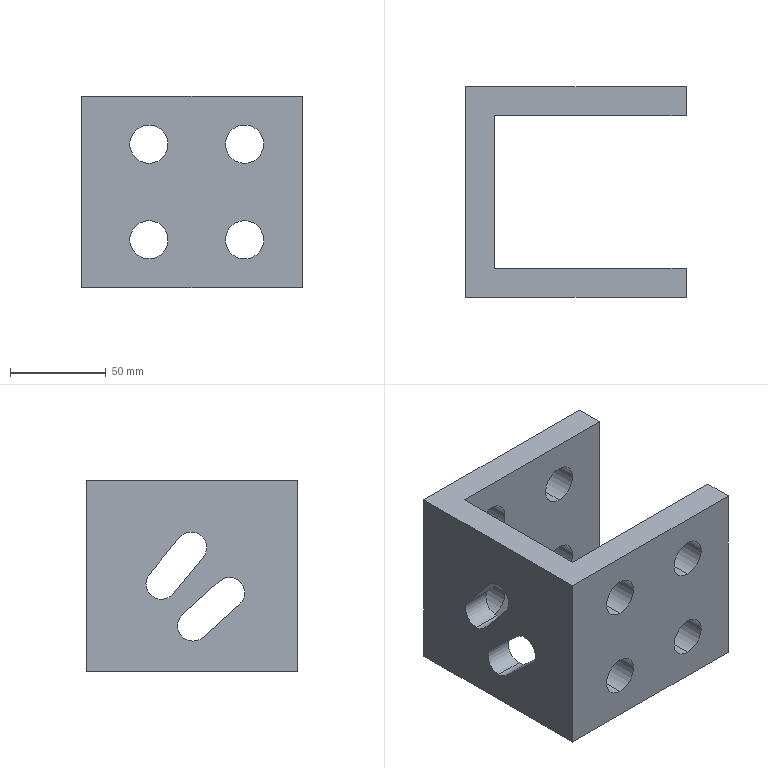Part | SolidWorks | features ICE 2, Extrusion 1 | 1 solid | 36 faces | box 115 x 110 x 100 mm | volume 409059 mm3 | cylinder 22 | plane 14 | commonest cylinder face diameters 20 x16 16.048 x3 16.141 x3
STEP:
#1=CARTESIAN_POINT('',(-15.,39.555,15.955));
#2=VERTEX_POINT('',#1);
#3=CARTESIAN_POINT('',(-15.,44.934,29.933));
#4=VERTEX_POINT('',#3);
#5=CARTESIAN_POINT('',(-15.,39.555,23.979));
#6=DIRECTION('',(1.,0.,0.));
#7=DIRECTION('',(0.,0.,-1.));
#8=AXIS2_PLACEMENT_3D('',#5,#6,#7);
#9=CIRCLE('',#8,8.024);
#10=EDGE_CURVE('',#2,#4,#9,.T.);
#11=ORIENTED_EDGE('',*,*,#10,.F.);
#12=CARTESIAN_POINT('',(0.,39.555,15.955));
#13=VERTEX_POINT('',#12);
#14=CARTESIAN_POINT('',(-500.,39.555,15.955));
#15=DIRECTION('',(1.,0.,0.));
#16=VECTOR('',#15,1000.);
#17=LINE('',#14,#16);
#18=EDGE_CURVE('',#2,#13,#17,.T.);
#19=ORIENTED_EDGE('',*,*,#18,.T.);
#20=CARTESIAN_POINT('',(0.,44.934,29.933));
#21=VERTEX_POINT('',#20);
#22=CARTESIAN_POINT('',(0.,39.555,23.979));
#23=DIRECTION('',(1.,0.,0.));
#24=DIRECTION('',(0.,0.,-1.));
#25=AXIS2_PLACEMENT_3D('',#22,#23,#24);
#26=CIRCLE('',#25,8.024);
#27=EDGE_CURVE('',#13,#21,#26,.T.);
#28=ORIENTED_EDGE('',*,*,#27,.T.);
#29=CARTESIAN_POINT('',(-500.,44.934,29.933));
#30=DIRECTION('',(1.,0.,0.));
#31=VECTOR('',#30,1000.);
#32=LINE('',#29,#31);
#33=EDGE_CURVE('',#4,#21,#32,.T.);
#34=ORIENTED_EDGE('',*,*,#33,.F.);
#35=EDGE_LOOP('',(#11,#19,#28,#34));
#36=FACE_OUTER_BOUND('',#35,.T.);
#37=CARTESIAN_POINT('',(-500.,39.555,23.979));
#38=DIRECTION('',(1.,0.,0.));
#39=DIRECTION('',(0.,0.,-1.));
#40=AXIS2_PLACEMENT_3D('',#37,#38,#39);
#41=CYLINDRICAL_SURFACE('',#40,8.024);
#42=ADVANCED_FACE('',(#36),#41,.F.);
#43=CARTESIAN_POINT('',(-15.,56.004,37.787));
#44=VERTEX_POINT('',#43);
#45=CARTESIAN_POINT('',(-15.,62.246,50.974));
#46=VERTEX_POINT('',#45);
#47=CARTESIAN_POINT('',(-15.,56.004,45.857));
#48=DIRECTION('',(1.,0.,0.));
#49=DIRECTION('',(0.,0.,-1.));
#50=AXIS2_PLACEMENT_3D('',#47,#48,#49);
#51=CIRCLE('',#50,8.071);
#52=EDGE_CURVE('',#44,#46,#51,.T.);
#53=ORIENTED_EDGE('',*,*,#52,.F.);
#54=CARTESIAN_POINT('',(0.,56.004,37.787));
#55=VERTEX_POINT('',#54);
#56=CARTESIAN_POINT('',(-500.,56.004,37.787));
#57=DIRECTION('',(1.,0.,0.));
#58=VECTOR('',#57,1000.);
#59=LINE('',#56,#58);
#60=EDGE_CURVE('',#44,#55,#59,.T.);
#61=ORIENTED_EDGE('',*,*,#60,.T.);
#62=CARTESIAN_POINT('',(0.,62.246,50.974));
#63=VERTEX_POINT('',#62);
#64=CARTESIAN_POINT('',(0.,56.004,45.857));
#65=DIRECTION('',(1.,0.,0.));
#66=DIRECTION('',(0.,0.,-1.));
#67=AXIS2_PLACEMENT_3D('',#64,#65,#66);
#68=CIRCLE('',#67,8.071);
#69=EDGE_CURVE('',#55,#63,#68,.T.);
#70=ORIENTED_EDGE('',*,*,#69,.T.);
#71=CARTESIAN_POINT('',(-500.,62.246,50.974));
#72=DIRECTION('',(1.,0.,0.));
#73=VECTOR('',#72,1000.);
#74=LINE('',#71,#73);
#75=EDGE_CURVE('',#46,#63,#74,.T.);
#76=ORIENTED_EDGE('',*,*,#75,.F.);
#77=EDGE_LOOP('',(#53,#61,#70,#76));
#78=FACE_OUTER_BOUND('',#77,.T.);
#79=CARTESIAN_POINT('',(-500.,56.004,45.857));
#80=DIRECTION('',(1.,0.,0.));
#81=DIRECTION('',(0.,0.,-1.));
#82=AXIS2_PLACEMENT_3D('',#79,#80,#81);
#83=CYLINDRICAL_SURFACE('',#82,8.071);
#84=ADVANCED_FACE('',(#78),#83,.F.);
#85=CARTESIAN_POINT('',(70.,80.,15.));
#86=VERTEX_POINT('',#85);
#87=CARTESIAN_POINT('',(70.,80.,35.));
#88=VERTEX_POINT('',#87);
#89=CARTESIAN_POINT('',(70.,80.,25.));
#90=DIRECTION('',(0.,1.,0.));
#91=DIRECTION('',(0.,0.,1.));
#92=AXIS2_PLACEMENT_3D('',#89,#90,#91);
#93=CIRCLE('',#92,10.);
#94=EDGE_CURVE('',#86,#88,#93,.T.);
#95=ORIENTED_EDGE('',*,*,#94,.F.);
#96=CARTESIAN_POINT('',(70.,95.,15.));
#97=VERTEX_POINT('',#96);
#98=CARTESIAN_POINT('',(70.,-405.,15.));
#99=DIRECTION('',(0.,1.,0.));
#100=VECTOR('',#99,1000.);
#101=LINE('',#98,#100);
#102=EDGE_CURVE('',#86,#97,#101,.T.);
#103=ORIENTED_EDGE('',*,*,#102,.T.);
#104=CARTESIAN_POINT('',(70.,95.,35.));
#105=VERTEX_POINT('',#104);
#106=CARTESIAN_POINT('',(70.,95.,25.));
#107=DIRECTION('',(0.,1.,0.));
#108=DIRECTION('',(0.,0.,1.));
#109=AXIS2_PLACEMENT_3D('',#106,#107,#108);
#110=CIRCLE('',#109,10.);
#111=EDGE_CURVE('',#97,#105,#110,.T.);
#112=ORIENTED_EDGE('',*,*,#111,.T.);
#113=CARTESIAN_POINT('',(70.,-405.,35.));
#114=DIRECTION('',(0.,1.,0.));
#115=VECTOR('',#114,1000.);
#116=LINE('',#113,#115);
#117=EDGE_CURVE('',#88,#105,#116,.T.);
#118=ORIENTED_EDGE('',*,*,#117,.F.);
#119=EDGE_LOOP('',(#95,#103,#112,#118));
#120=FACE_OUTER_BOUND('',#119,.T.);
#121=CARTESIAN_POINT('',(70.,-405.,25.));
#122=DIRECTION('',(0.,1.,0.));
#123=DIRECTION('',(0.,0.,1.));
#124=AXIS2_PLACEMENT_3D('',#121,#122,#123);
#125=CYLINDRICAL_SURFACE('',#124,10.);
#126=ADVANCED_FACE('',(#120),#125,.F.);
#127=CARTESIAN_POINT('',(20.,80.,65.));
#128=VERTEX_POINT('',#127);
#129=CARTESIAN_POINT('',(20.,80.,85.));
#130=VERTEX_POINT('',#129);
#131=CARTESIAN_POINT('',(20.,80.,75.));
#132=DIRECTION('',(0.,1.,0.));
#133=DIRECTION('',(0.,0.,1.));
#134=AXIS2_PLACEMENT_3D('',#131,#132,#133);
#135=CIRCLE('',#134,10.);
#136=EDGE_CURVE('',#128,#130,#135,.T.);
#137=ORIENTED_EDGE('',*,*,#136,.F.);
#138=CARTESIAN_POINT('',(20.,95.,65.));
#139=VERTEX_POINT('',#138);
#140=CARTESIAN_POINT('',(20.,-405.,65.));
#141=DIRECTION('',(0.,1.,0.));
#142=VECTOR('',#141,1000.);
#143=LINE('',#140,#142);
#144=EDGE_CURVE('',#128,#139,#143,.T.);
#145=ORIENTED_EDGE('',*,*,#144,.T.);
#146=CARTESIAN_POINT('',(20.,95.,85.));
#147=VERTEX_POINT('',#146);
#148=CARTESIAN_POINT('',(20.,95.,75.));
#149=DIRECTION('',(0.,1.,0.));
#150=DIRECTION('',(0.,0.,1.));
#151=AXIS2_PLACEMENT_3D('',#148,#149,#150);
#152=CIRCLE('',#151,10.);
#153=EDGE_CURVE('',#139,#147,#152,.T.);
#154=ORIENTED_EDGE('',*,*,#153,.T.);
#155=CARTESIAN_POINT('',(20.,-405.,85.));
#156=DIRECTION('',(0.,1.,0.));
#157=VECTOR('',#156,1000.);
#158=LINE('',#155,#157);
#159=EDGE_CURVE('',#130,#147,#158,.T.);
#160=ORIENTED_EDGE('',*,*,#159,.F.);
#161=EDGE_LOOP('',(#137,#145,#154,#160));
#162=FACE_OUTER_BOUND('',#161,.T.);
#163=CARTESIAN_POINT('',(20.,-405.,75.));
#164=DIRECTION('',(0.,1.,0.));
#165=DIRECTION('',(0.,0.,1.));
#166=AXIS2_PLACEMENT_3D('',#163,#164,#165);
#167=CYLINDRICAL_SURFACE('',#166,10.);
#168=ADVANCED_FACE('',(#162),#167,.F.);
#169=CARTESIAN_POINT('',(70.,80.,65.));
#170=VERTEX_POINT('',#169);
#171=CARTESIAN_POINT('',(70.,80.,85.));
#172=VERTEX_POINT('',#171);
#173=CARTESIAN_POINT('',(70.,80.,75.));
#174=DIRECTION('',(0.,1.,0.));
#175=DIRECTION('',(0.,0.,1.));
#176=AXIS2_PLACEMENT_3D('',#173,#174,#175);
#177=CIRCLE('',#176,10.);
#178=EDGE_CURVE('',#170,#172,#177,.T.);
#179=ORIENTED_EDGE('',*,*,#178,.F.);
#180=CARTESIAN_POINT('',(70.,95.,65.));
#181=VERTEX_POINT('',#180);
#182=CARTESIAN_POINT('',(70.,-405.,65.));
#183=DIRECTION('',(0.,1.,0.));
#184=VECTOR('',#183,1000.);
#185=LINE('',#182,#184);
#186=EDGE_CURVE('',#170,#181,#185,.T.);
#187=ORIENTED_EDGE('',*,*,#186,.T.);
#188=CARTESIAN_POINT('',(70.,95.,85.));
#189=VERTEX_POINT('',#188);
#190=CARTESIAN_POINT('',(70.,95.,75.));
#191=DIRECTION('',(0.,1.,0.));
#192=DIRECTION('',(0.,0.,1.));
#193=AXIS2_PLACEMENT_3D('',#190,#191,#192);
#194=CIRCLE('',#193,10.);
#195=EDGE_CURVE('',#181,#189,#194,.T.);
#196=ORIENTED_EDGE('',*,*,#195,.T.);
#197=CARTESIAN_POINT('',(70.,-405.,85.));
#198=DIRECTION('',(0.,1.,0.));
#199=VECTOR('',#198,1000.);
#200=LINE('',#197,#199);
#201=EDGE_CURVE('',#172,#189,#200,.T.);
#202=ORIENTED_EDGE('',*,*,#201,.F.);
#203=EDGE_LOOP('',(#179,#187,#196,#202));
#204=FACE_OUTER_BOUND('',#203,.T.);
#205=CARTESIAN_POINT('',(70.,-405.,75.));
#206=DIRECTION('',(0.,1.,0.));
#207=DIRECTION('',(0.,0.,1.));
#208=AXIS2_PLACEMENT_3D('',#205,#206,#207);
#209=CYLINDRICAL_SURFACE('',#208,10.);
#210=ADVANCED_FACE('',(#204),#209,.F.);
#211=CARTESIAN_POINT('',(20.,80.,15.));
#212=VERTEX_POINT('',#211);
#213=CARTESIAN_POINT('',(20.,80.,35.));
#214=VERTEX_POINT('',#213);
#215=CARTESIAN_POINT('',(20.,80.,25.));
#216=DIRECTION('',(0.,1.,0.));
#217=DIRECTION('',(0.,0.,1.));
#218=AXIS2_PLACEMENT_3D('',#215,#216,#217);
#219=CIRCLE('',#218,10.);
#220=EDGE_CURVE('',#212,#214,#219,.T.);
#221=ORIENTED_EDGE('',*,*,#220,.F.);
#222=CARTESIAN_POINT('',(20.,95.,15.));
#223=VERTEX_POINT('',#222);
#224=CARTESIAN_POINT('',(20.,-405.,15.));
#225=DIRECTION('',(0.,1.,0.));
#226=VECTOR('',#225,1000.);
#227=LINE('',#224,#226);
#228=EDGE_CURVE('',#212,#223,#227,.T.);
#229=ORIENTED_EDGE('',*,*,#228,.T.);
#230=CARTESIAN_POINT('',(20.,95.,35.));
#231=VERTEX_POINT('',#230);
#232=CARTESIAN_POINT('',(20.,95.,25.));
#233=DIRECTION('',(0.,1.,0.));
#234=DIRECTION('',(0.,0.,1.));
#235=AXIS2_PLACEMENT_3D('',#232,#233,#234);
#236=CIRCLE('',#235,10.);
#237=EDGE_CURVE('',#223,#231,#236,.T.);
#238=ORIENTED_EDGE('',*,*,#237,.T.);
#239=CARTESIAN_POINT('',(20.,-405.,35.));
#240=DIRECTION('',(0.,1.,0.));
#241=VECTOR('',#240,1000.);
#242=LINE('',#239,#241);
#243=EDGE_CURVE('',#214,#231,#242,.T.);
#244=ORIENTED_EDGE('',*,*,#243,.F.);
#245=EDGE_LOOP('',(#221,#229,#238,#244));
#246=FACE_OUTER_BOUND('',#245,.T.);
#247=CARTESIAN_POINT('',(20.,-405.,25.));
#248=DIRECTION('',(0.,1.,0.));
#249=DIRECTION('',(0.,0.,1.));
#250=AXIS2_PLACEMENT_3D('',#247,#248,#249);
#251=CYLINDRICAL_SURFACE('',#250,10.);
#252=ADVANCED_FACE('',(#246),#251,.F.);
#253=CARTESIAN_POINT('',(70.,-15.,15.));
#254=VERTEX_POINT('',#253);
#255=CARTESIAN_POINT('',(70.,-15.,35.));
#256=VERTEX_POINT('',#255);
#257=CARTESIAN_POINT('',(70.,-15.,25.));
#258=DIRECTION('',(0.,1.,0.));
#259=DIRECTION('',(0.,0.,1.));
#260=AXIS2_PLACEMENT_3D('',#257,#258,#259);
#261=CIRCLE('',#260,10.);
#262=EDGE_CURVE('',#254,#256,#261,.T.);
#263=ORIENTED_EDGE('',*,*,#262,.F.);
#264=CARTESIAN_POINT('',(70.,0.,15.));
#265=VERTEX_POINT('',#264);
#266=CARTESIAN_POINT('',(70.,-405.,15.));
#267=DIRECTION('',(0.,1.,0.));
#268=VECTOR('',#267,1000.);
#269=LINE('',#266,#268);
#270=EDGE_CURVE('',#254,#265,#269,.T.);
#271=ORIENTED_EDGE('',*,*,#270,.T.);
#272=CARTESIAN_POINT('',(70.,0.,35.));
#273=VERTEX_POINT('',#272);
#274=CARTESIAN_POINT('',(70.,0.,25.));
#275=DIRECTION('',(0.,-1.,0.));
#276=DIRECTION('',(0.,0.,-1.));
#277=AXIS2_PLACEMENT_3D('',#274,#275,#276);
#278=CIRCLE('',#277,10.);
#279=EDGE_CURVE('',#273,#265,#278,.T.);
#280=ORIENTED_EDGE('',*,*,#279,.F.);
#281=CARTESIAN_POINT('',(70.,-405.,35.));
#282=DIRECTION('',(0.,1.,0.));
#283=VECTOR('',#282,1000.);
#284=LINE('',#281,#283);
#285=EDGE_CURVE('',#256,#273,#284,.T.);
#286=ORIENTED_EDGE('',*,*,#285,.F.);
#287=EDGE_LOOP('',(#263,#271,#280,#286));
#288=FACE_OUTER_BOUND('',#287,.T.);
#289=CARTESIAN_POINT('',(70.,-405.,25.));
#290=DIRECTION('',(0.,1.,0.));
#291=DIRECTION('',(0.,0.,1.));
#292=AXIS2_PLACEMENT_3D('',#289,#290,#291);
#293=CYLINDRICAL_SURFACE('',#292,10.);
#294=ADVANCED_FACE('',(#288),#293,.F.);
#295=CARTESIAN_POINT('',(20.,-15.,65.));
#296=VERTEX_POINT('',#295);
#297=CARTESIAN_POINT('',(20.,-15.,85.));
#298=VERTEX_POINT('',#297);
#299=CARTESIAN_POINT('',(20.,-15.,75.));
#300=DIRECTION('',(0.,1.,0.));
#301=DIRECTION('',(0.,0.,1.));
#302=AXIS2_PLACEMENT_3D('',#299,#300,#301);
#303=CIRCLE('',#302,10.);
#304=EDGE_CURVE('',#296,#298,#303,.T.);
#305=ORIENTED_EDGE('',*,*,#304,.F.);
#306=CARTESIAN_POINT('',(20.,0.,65.));
#307=VERTEX_POINT('',#306);
#308=CARTESIAN_POINT('',(20.,-405.,65.));
#309=DIRECTION('',(0.,1.,0.));
#310=VECTOR('',#309,1000.);
#311=LINE('',#308,#310);
#312=EDGE_CURVE('',#296,#307,#311,.T.);
#313=ORIENTED_EDGE('',*,*,#312,.T.);
#314=CARTESIAN_POINT('',(20.,0.,85.));
#315=VERTEX_POINT('',#314);
#316=CARTESIAN_POINT('',(20.,0.,75.));
#317=DIRECTION('',(0.,-1.,0.));
#318=DIRECTION('',(0.,0.,-1.));
#319=AXIS2_PLACEMENT_3D('',#316,#317,#318);
#320=CIRCLE('',#319,10.);
#321=EDGE_CURVE('',#315,#307,#320,.T.);
#322=ORIENTED_EDGE('',*,*,#321,.F.);
#323=CARTESIAN_POINT('',(20.,-405.,85.));
#324=DIRECTION('',(0.,1.,0.));
#325=VECTOR('',#324,1000.);
#326=LINE('',#323,#325);
#327=EDGE_CURVE('',#298,#315,#326,.T.);
#328=ORIENTED_EDGE('',*,*,#327,.F.);
#329=EDGE_LOOP('',(#305,#313,#322,#328));
#330=FACE_OUTER_BOUND('',#329,.T.);
#331=CARTESIAN_POINT('',(20.,-405.,75.));
#332=DIRECTION('',(0.,1.,0.));
#333=DIRECTION('',(0.,0.,1.));
#334=AXIS2_PLACEMENT_3D('',#331,#332,#333);
#335=CYLINDRICAL_SURFACE('',#334,10.);
#336=ADVANCED_FACE('',(#330),#335,.F.);
#337=CARTESIAN_POINT('',(70.,-15.,65.));
#338=VERTEX_POINT('',#337);
#339=CARTESIAN_POINT('',(70.,-15.,85.));
#340=VERTEX_POINT('',#339);
#341=CARTESIAN_POINT('',(70.,-15.,75.));
#342=DIRECTION('',(0.,1.,0.));
#343=DIRECTION('',(0.,0.,1.));
#344=AXIS2_PLACEMENT_3D('',#341,#342,#343);
#345=CIRCLE('',#344,10.);
#346=EDGE_CURVE('',#338,#340,#345,.T.);
#347=ORIENTED_EDGE('',*,*,#346,.F.);
#348=CARTESIAN_POINT('',(70.,0.,65.));
#349=VERTEX_POINT('',#348);
#350=CARTESIAN_POINT('',(70.,-405.,65.));
#351=DIRECTION('',(0.,1.,0.));
#352=VECTOR('',#351,1000.);
#353=LINE('',#350,#352);
#354=EDGE_CURVE('',#338,#349,#353,.T.);
#355=ORIENTED_EDGE('',*,*,#354,.T.);
#356=CARTESIAN_POINT('',(70.,0.,85.));
#357=VERTEX_POINT('',#356);
#358=CARTESIAN_POINT('',(70.,0.,75.));
#359=DIRECTION('',(0.,-1.,0.));
#360=DIRECTION('',(0.,0.,-1.));
#361=AXIS2_PLACEMENT_3D('',#358,#359,#360);
#362=CIRCLE('',#361,10.);
#363=EDGE_CURVE('',#357,#349,#362,.T.);
#364=ORIENTED_EDGE('',*,*,#363,.F.);
#365=CARTESIAN_POINT('',(70.,-405.,85.));
#366=DIRECTION('',(0.,1.,0.));
#367=VECTOR('',#366,1000.);
#368=LINE('',#365,#367);
#369=EDGE_CURVE('',#340,#357,#368,.T.);
#370=ORIENTED_EDGE('',*,*,#369,.F.);
#371=EDGE_LOOP('',(#347,#355,#364,#370));
#372=FACE_OUTER_BOUND('',#371,.T.);
#373=CARTESIAN_POINT('',(70.,-405.,75.));
#374=DIRECTION('',(0.,1.,0.));
#375=DIRECTION('',(0.,0.,1.));
#376=AXIS2_PLACEMENT_3D('',#373,#374,#375);
#377=CYLINDRICAL_SURFACE('',#376,10.);
#378=ADVANCED_FACE('',(#372),#377,.F.);
#379=CARTESIAN_POINT('',(20.,-15.,15.));
#380=VERTEX_POINT('',#379);
#381=CARTESIAN_POINT('',(20.,-15.,35.));
#382=VERTEX_POINT('',#381);
#383=CARTESIAN_POINT('',(20.,-15.,25.));
#384=DIRECTION('',(0.,1.,0.));
#385=DIRECTION('',(0.,0.,1.));
#386=AXIS2_PLACEMENT_3D('',#383,#384,#385);
#387=CIRCLE('',#386,10.);
#388=EDGE_CURVE('',#380,#382,#387,.T.);
#389=ORIENTED_EDGE('',*,*,#388,.F.);
#390=CARTESIAN_POINT('',(20.,0.,15.));
#391=VERTEX_POINT('',#390);
#392=CARTESIAN_POINT('',(20.,-405.,15.));
#393=DIRECTION('',(0.,1.,0.));
#394=VECTOR('',#393,1000.);
#395=LINE('',#392,#394);
#396=EDGE_CURVE('',#380,#391,#395,.T.);
#397=ORIENTED_EDGE('',*,*,#396,.T.);
#398=CARTESIAN_POINT('',(20.,0.,35.));
#399=VERTEX_POINT('',#398);
#400=CARTESIAN_POINT('',(20.,0.,25.));
#401=DIRECTION('',(0.,-1.,0.));
#402=DIRECTION('',(0.,0.,-1.));
#403=AXIS2_PLACEMENT_3D('',#400,#401,#402);
#404=CIRCLE('',#403,10.);
#405=EDGE_CURVE('',#399,#391,#404,.T.);
#406=ORIENTED_EDGE('',*,*,#405,.F.);
#407=CARTESIAN_POINT('',(20.,-405.,35.));
#408=DIRECTION('',(0.,1.,0.));
#409=VECTOR('',#408,1000.);
#410=LINE('',#407,#409);
#411=EDGE_CURVE('',#382,#399,#410,.T.);
#412=ORIENTED_EDGE('',*,*,#411,.F.);
#413=EDGE_LOOP('',(#389,#397,#406,#412));
#414=FACE_OUTER_BOUND('',#413,.T.);
#415=CARTESIAN_POINT('',(20.,-405.,25.));
#416=DIRECTION('',(0.,1.,0.));
#417=DIRECTION('',(0.,0.,1.));
#418=AXIS2_PLACEMENT_3D('',#415,#416,#417);
#419=CYLINDRICAL_SURFACE('',#418,10.);
#420=ADVANCED_FACE('',(#414),#419,.F.);
#421=CARTESIAN_POINT('',(0.,15.111,35.249));
#422=VERTEX_POINT('',#421);
#423=CARTESIAN_POINT('',(0.,34.175,18.025));
#424=VERTEX_POINT('',#423);
#425=CARTESIAN_POINT('',(0.,15.111,35.249));
#426=DIRECTION('',(0.,0.742,-0.6704));
#427=VECTOR('',#426,1000.);
#428=LINE('',#425,#427);
#429=EDGE_CURVE('',#422,#424,#428,.T.);
#430=ORIENTED_EDGE('',*,*,#429,.F.);
#431=CARTESIAN_POINT('',(0.,25.87,47.157));
#432=VERTEX_POINT('',#431);
#433=CARTESIAN_POINT('',(0.,20.49,41.203));
#434=DIRECTION('',(1.,0.,0.));
#435=DIRECTION('',(0.,0.,-1.));
#436=AXIS2_PLACEMENT_3D('',#433,#434,#435);
#437=CIRCLE('',#436,8.024);
#438=EDGE_CURVE('',#432,#422,#437,.T.);
#439=ORIENTED_EDGE('',*,*,#438,.F.);
#440=CARTESIAN_POINT('',(0.,25.87,47.157));
#441=DIRECTION('',(0.,-0.742,0.6704));
#442=VECTOR('',#441,1000.);
#443=LINE('',#440,#442);
#444=EDGE_CURVE('',#21,#432,#443,.T.);
#445=ORIENTED_EDGE('',*,*,#444,.F.);
#446=ORIENTED_EDGE('',*,*,#27,.F.);
#447=CARTESIAN_POINT('',(0.,39.555,23.979));
#448=DIRECTION('',(1.,0.,0.));
#449=DIRECTION('',(0.,0.,-1.));
#450=AXIS2_PLACEMENT_3D('',#447,#448,#449);
#451=CIRCLE('',#450,8.024);
#452=EDGE_CURVE('',#424,#13,#451,.T.);
#453=ORIENTED_EDGE('',*,*,#452,.F.);
#454=EDGE_LOOP('',(#430,#439,#445,#446,#453));
#455=FACE_BOUND('',#454,.T.);
#456=CARTESIAN_POINT('',(0.,34.175,59.757));
#457=VERTEX_POINT('',#456);
#458=CARTESIAN_POINT('',(0.,49.762,40.741));
#459=VERTEX_POINT('',#458);
#460=CARTESIAN_POINT('',(0.,34.175,59.757));
#461=DIRECTION('',(0.,0.6339,-0.7734));
#462=VECTOR('',#461,1000.);
#463=LINE('',#460,#462);
#464=EDGE_CURVE('',#457,#459,#463,.T.);
#465=ORIENTED_EDGE('',*,*,#464,.F.);
#466=CARTESIAN_POINT('',(0.,46.659,69.989));
#467=VERTEX_POINT('',#466);
#468=CARTESIAN_POINT('',(0.,40.417,64.873));
#469=DIRECTION('',(1.,0.,0.));
#470=DIRECTION('',(0.,0.,-1.));
#471=AXIS2_PLACEMENT_3D('',#468,#469,#470);
#472=CIRCLE('',#471,8.071);
#473=EDGE_CURVE('',#467,#457,#472,.T.);
#474=ORIENTED_EDGE('',*,*,#473,.F.);
#475=CARTESIAN_POINT('',(0.,46.659,69.989));
#476=DIRECTION('',(0.,-0.6339,0.7734));
#477=VECTOR('',#476,1000.);
#478=LINE('',#475,#477);
#479=EDGE_CURVE('',#63,#467,#478,.T.);
#480=ORIENTED_EDGE('',*,*,#479,.F.);
#481=ORIENTED_EDGE('',*,*,#69,.F.);
#482=CARTESIAN_POINT('',(0.,56.004,45.857));
#483=DIRECTION('',(1.,0.,0.));
#484=DIRECTION('',(0.,0.,-1.));
#485=AXIS2_PLACEMENT_3D('',#482,#483,#484);
#486=CIRCLE('',#485,8.071);
#487=EDGE_CURVE('',#459,#55,#486,.T.);
#488=ORIENTED_EDGE('',*,*,#487,.F.);
#489=EDGE_LOOP('',(#465,#474,#480,#481,#488));
#490=FACE_BOUND('',#489,.T.);
#491=CARTESIAN_POINT('',(0.,0.,0.));
#492=VERTEX_POINT('',#491);
#493=CARTESIAN_POINT('',(0.,80.,0.));
#494=VERTEX_POINT('',#493);
#495=CARTESIAN_POINT('',(0.,0.,0.));
#496=DIRECTION('',(0.,1.,0.));
#497=VECTOR('',#496,1000.);
#498=LINE('',#495,#497);
#499=EDGE_CURVE('',#492,#494,#498,.T.);
#500=ORIENTED_EDGE('',*,*,#499,.T.);
#501=CARTESIAN_POINT('',(0.,80.,100.));
#502=VERTEX_POINT('',#501);
#503=CARTESIAN_POINT('',(0.,80.,100.));
#504=DIRECTION('',(0.,0.,-1.));
#505=VECTOR('',#504,1000.);
#506=LINE('',#503,#505);
#507=EDGE_CURVE('',#502,#494,#506,.T.);
#508=ORIENTED_EDGE('',*,*,#507,.F.);
#509=CARTESIAN_POINT('',(0.,0.,100.));
#510=VERTEX_POINT('',#509);
#511=CARTESIAN_POINT('',(0.,0.,100.));
#512=DIRECTION('',(0.,1.,0.));
#513=VECTOR('',#512,1000.);
#514=LINE('',#511,#513);
#515=EDGE_CURVE('',#510,#502,#514,.T.);
#516=ORIENTED_EDGE('',*,*,#515,.F.);
#517=CARTESIAN_POINT('',(0.,0.,100.));
#518=DIRECTION('',(0.,0.,-1.));
#519=VECTOR('',#518,1000.);
#520=LINE('',#517,#519);
#521=EDGE_CURVE('',#510,#492,#520,.T.);
#522=ORIENTED_EDGE('',*,*,#521,.T.);
#523=EDGE_LOOP('',(#500,#508,#516,#522));
#524=FACE_OUTER_BOUND('',#523,.T.);
#525=CARTESIAN_POINT('',(0.,0.,100.));
#526=DIRECTION('',(-1.,0.,0.));
#527=DIRECTION('',(0.,0.,1.));
#528=AXIS2_PLACEMENT_3D('',#525,#526,#527);
#529=PLANE('',#528);
#530=ADVANCED_FACE('',(#455,#490,#524),#529,.F.);
#531=CARTESIAN_POINT('',(70.,80.,25.));
#532=DIRECTION('',(0.,1.,0.));
#533=DIRECTION('',(0.,0.,1.));
#534=AXIS2_PLACEMENT_3D('',#531,#532,#533);
#535=CIRCLE('',#534,10.);
#536=EDGE_CURVE('',#88,#86,#535,.T.);
#537=ORIENTED_EDGE('',*,*,#536,.T.);
#538=ORIENTED_EDGE('',*,*,#94,.T.);
#539=EDGE_LOOP('',(#537,#538));
#540=FACE_BOUND('',#539,.T.);
#541=CARTESIAN_POINT('',(20.,80.,75.));
#542=DIRECTION('',(0.,1.,0.));
#543=DIRECTION('',(0.,0.,1.));
#544=AXIS2_PLACEMENT_3D('',#541,#542,#543);
#545=CIRCLE('',#544,10.);
#546=EDGE_CURVE('',#130,#128,#545,.T.);
#547=ORIENTED_EDGE('',*,*,#546,.T.);
#548=ORIENTED_EDGE('',*,*,#136,.T.);
#549=EDGE_LOOP('',(#547,#548));
#550=FACE_BOUND('',#549,.T.);
#551=CARTESIAN_POINT('',(70.,80.,75.));
#552=DIRECTION('',(0.,1.,0.));
#553=DIRECTION('',(0.,0.,1.));
#554=AXIS2_PLACEMENT_3D('',#551,#552,#553);
#555=CIRCLE('',#554,10.);
#556=EDGE_CURVE('',#172,#170,#555,.T.);
#557=ORIENTED_EDGE('',*,*,#556,.T.);
#558=ORIENTED_EDGE('',*,*,#178,.T.);
#559=EDGE_LOOP('',(#557,#558));
#560=FACE_BOUND('',#559,.T.);
#561=CARTESIAN_POINT('',(20.,80.,25.));
#562=DIRECTION('',(0.,1.,0.));
#563=DIRECTION('',(0.,0.,1.));
#564=AXIS2_PLACEMENT_3D('',#561,#562,#563);
#565=CIRCLE('',#564,10.);
#566=EDGE_CURVE('',#214,#212,#565,.T.);
#567=ORIENTED_EDGE('',*,*,#566,.T.);
#568=ORIENTED_EDGE('',*,*,#220,.T.);
#569=EDGE_LOOP('',(#567,#568));
#570=FACE_BOUND('',#569,.T.);
#571=CARTESIAN_POINT('',(100.,80.,0.));
#572=VERTEX_POINT('',#571);
#573=CARTESIAN_POINT('',(0.,80.,0.));
#574=DIRECTION('',(1.,0.,0.));
#575=VECTOR('',#574,1000.);
#576=LINE('',#573,#575);
#577=EDGE_CURVE('',#494,#572,#576,.T.);
#578=ORIENTED_EDGE('',*,*,#577,.T.);
#579=CARTESIAN_POINT('',(100.,80.,100.));
#580=VERTEX_POINT('',#579);
#581=CARTESIAN_POINT('',(100.,80.,100.));
#582=DIRECTION('',(0.,0.,-1.));
#583=VECTOR('',#582,1000.);
#584=LINE('',#581,#583);
#585=EDGE_CURVE('',#580,#572,#584,.T.);
#586=ORIENTED_EDGE('',*,*,#585,.F.);
#587=CARTESIAN_POINT('',(0.,80.,100.));
#588=DIRECTION('',(1.,0.,0.));
#589=VECTOR('',#588,1000.);
#590=LINE('',#587,#589);
#591=EDGE_CURVE('',#502,#580,#590,.T.);
#592=ORIENTED_EDGE('',*,*,#591,.F.);
#593=ORIENTED_EDGE('',*,*,#507,.T.);
#594=EDGE_LOOP('',(#578,#586,#592,#593));
#595=FACE_OUTER_BOUND('',#594,.T.);
#596=CARTESIAN_POINT('',(0.,80.,100.));
#597=DIRECTION('',(0.,1.,0.));
#598=DIRECTION('',(0.,0.,1.));
#599=AXIS2_PLACEMENT_3D('',#596,#597,#598);
#600=PLANE('',#599);
#601=ADVANCED_FACE('',(#540,#550,#560,#570,#595),#600,.F.);
#602=CARTESIAN_POINT('',(100.,95.,0.));
#603=VERTEX_POINT('',#602);
#604=CARTESIAN_POINT('',(100.,95.,0.));
#605=DIRECTION('',(0.,1.,0.));
#606=VECTOR('',#605,1000.);
#607=LINE('',#604,#606);
#608=EDGE_CURVE('',#572,#603,#607,.T.);
#609=ORIENTED_EDGE('',*,*,#608,.T.);
#610=CARTESIAN_POINT('',(100.,95.,100.));
#611=VERTEX_POINT('',#610);
#612=CARTESIAN_POINT('',(100.,95.,100.));
#613=DIRECTION('',(0.,0.,-1.));
#614=VECTOR('',#613,1000.);
#615=LINE('',#612,#614);
#616=EDGE_CURVE('',#611,#603,#615,.T.);
#617=ORIENTED_EDGE('',*,*,#616,.F.);
#618=CARTESIAN_POINT('',(100.,95.,100.));
#619=DIRECTION('',(0.,1.,0.));
#620=VECTOR('',#619,1000.);
#621=LINE('',#618,#620);
#622=EDGE_CURVE('',#580,#611,#621,.T.);
#623=ORIENTED_EDGE('',*,*,#622,.F.);
#624=ORIENTED_EDGE('',*,*,#585,.T.);
#625=EDGE_LOOP('',(#609,#617,#623,#624));
#626=FACE_OUTER_BOUND('',#625,.T.);
#627=CARTESIAN_POINT('',(100.,95.,100.));
#628=DIRECTION('',(-1.,0.,0.));
#629=DIRECTION('',(0.,0.,1.));
#630=AXIS2_PLACEMENT_3D('',#627,#628,#629);
#631=PLANE('',#630);
#632=ADVANCED_FACE('',(#626),#631,.F.);
#633=CARTESIAN_POINT('',(70.,95.,25.));
#634=DIRECTION('',(0.,1.,0.));
#635=DIRECTION('',(0.,0.,1.));
#636=AXIS2_PLACEMENT_3D('',#633,#634,#635);
#637=CIRCLE('',#636,10.);
#638=EDGE_CURVE('',#105,#97,#637,.T.);
#639=ORIENTED_EDGE('',*,*,#638,.F.);
#640=ORIENTED_EDGE('',*,*,#111,.F.);
#641=EDGE_LOOP('',(#639,#640));
#642=FACE_BOUND('',#641,.T.);
#643=CARTESIAN_POINT('',(20.,95.,75.));
#644=DIRECTION('',(0.,1.,0.));
#645=DIRECTION('',(0.,0.,1.));
#646=AXIS2_PLACEMENT_3D('',#643,#644,#645);
#647=CIRCLE('',#646,10.);
#648=EDGE_CURVE('',#147,#139,#647,.T.);
#649=ORIENTED_EDGE('',*,*,#648,.F.);
#650=ORIENTED_EDGE('',*,*,#153,.F.);
#651=EDGE_LOOP('',(#649,#650));
#652=FACE_BOUND('',#651,.T.);
#653=CARTESIAN_POINT('',(70.,95.,75.));
#654=DIRECTION('',(0.,1.,0.));
#655=DIRECTION('',(0.,0.,1.));
#656=AXIS2_PLACEMENT_3D('',#653,#654,#655);
#657=CIRCLE('',#656,10.);
#658=EDGE_CURVE('',#189,#181,#657,.T.);
#659=ORIENTED_EDGE('',*,*,#658,.F.);
#660=ORIENTED_EDGE('',*,*,#195,.F.);
#661=EDGE_LOOP('',(#659,#660));
#662=FACE_BOUND('',#661,.T.);
#663=CARTESIAN_POINT('',(20.,95.,25.));
#664=DIRECTION('',(0.,1.,0.));
#665=DIRECTION('',(0.,0.,1.));
#666=AXIS2_PLACEMENT_3D('',#663,#664,#665);
#667=CIRCLE('',#666,10.);
#668=EDGE_CURVE('',#231,#223,#667,.T.);
#669=ORIENTED_EDGE('',*,*,#668,.F.);
#670=ORIENTED_EDGE('',*,*,#237,.F.);
#671=EDGE_LOOP('',(#669,#670));
#672=FACE_BOUND('',#671,.T.);
#673=CARTESIAN_POINT('',(-15.,95.,0.));
#674=VERTEX_POINT('',#673);
#675=CARTESIAN_POINT('',(-15.,95.,0.));
#676=DIRECTION('',(-1.,0.,0.));
#677=VECTOR('',#676,1000.);
#678=LINE('',#675,#677);
#679=EDGE_CURVE('',#603,#674,#678,.T.);
#680=ORIENTED_EDGE('',*,*,#679,.T.);
#681=CARTESIAN_POINT('',(-15.,95.,100.));
#682=VERTEX_POINT('',#681);
#683=CARTESIAN_POINT('',(-15.,95.,100.));
#684=DIRECTION('',(0.,0.,-1.));
#685=VECTOR('',#684,1000.);
#686=LINE('',#683,#685);
#687=EDGE_CURVE('',#682,#674,#686,.T.);
#688=ORIENTED_EDGE('',*,*,#687,.F.);
#689=CARTESIAN_POINT('',(-15.,95.,100.));
#690=DIRECTION('',(-1.,0.,0.));
#691=VECTOR('',#690,1000.);
#692=LINE('',#689,#691);
#693=EDGE_CURVE('',#611,#682,#692,.T.);
#694=ORIENTED_EDGE('',*,*,#693,.F.);
#695=ORIENTED_EDGE('',*,*,#616,.T.);
#696=EDGE_LOOP('',(#680,#688,#694,#695));
#697=FACE_OUTER_BOUND('',#696,.T.);
#698=CARTESIAN_POINT('',(-15.,95.,100.));
#699=DIRECTION('',(0.,-1.,0.));
#700=DIRECTION('',(0.,0.,-1.));
#701=AXIS2_PLACEMENT_3D('',#698,#699,#700);
#702=PLANE('',#701);
#703=ADVANCED_FACE('',(#642,#652,#662,#672,#697),#702,.F.);
#704=CARTESIAN_POINT('',(-15.,25.87,47.157));
#705=VERTEX_POINT('',#704);
#706=CARTESIAN_POINT('',(-15.,-22.918,91.236));
#707=DIRECTION('',(0.,-0.742,0.6704));
#708=VECTOR('',#707,1000.);
#709=LINE('',#706,#708);
#710=EDGE_CURVE('',#4,#705,#709,.T.);
#711=ORIENTED_EDGE('',*,*,#710,.T.);
#712=CARTESIAN_POINT('',(-15.,15.111,35.249));
#713=VERTEX_POINT('',#712);
#714=CARTESIAN_POINT('',(-15.,20.49,41.203));
#715=DIRECTION('',(1.,0.,0.));
#716=DIRECTION('',(0.,0.,-1.));
#717=AXIS2_PLACEMENT_3D('',#714,#715,#716);
#718=CIRCLE('',#717,8.024);
#719=EDGE_CURVE('',#705,#713,#718,.T.);
#720=ORIENTED_EDGE('',*,*,#719,.T.);
#721=CARTESIAN_POINT('',(-15.,34.175,18.025));
#722=VERTEX_POINT('',#721);
#723=CARTESIAN_POINT('',(-15.,-33.677,79.328));
#724=DIRECTION('',(0.,0.742,-0.6704));
#725=VECTOR('',#724,1000.);
#726=LINE('',#723,#725);
#727=EDGE_CURVE('',#713,#722,#726,.T.);
#728=ORIENTED_EDGE('',*,*,#727,.T.);
#729=CARTESIAN_POINT('',(-15.,39.555,23.979));
#730=DIRECTION('',(1.,0.,0.));
#731=DIRECTION('',(0.,0.,-1.));
#732=AXIS2_PLACEMENT_3D('',#729,#730,#731);
#733=CIRCLE('',#732,8.024);
#734=EDGE_CURVE('',#722,#2,#733,.T.);
#735=ORIENTED_EDGE('',*,*,#734,.T.);
#736=ORIENTED_EDGE('',*,*,#10,.T.);
#737=EDGE_LOOP('',(#711,#720,#728,#735,#736));
#738=FACE_BOUND('',#737,.T.);
#739=CARTESIAN_POINT('',(-15.,46.659,69.989));
#740=VERTEX_POINT('',#739);
#741=CARTESIAN_POINT('',(-15.,7.167,118.17));
#742=DIRECTION('',(0.,-0.6339,0.7734));
#743=VECTOR('',#742,1000.);
#744=LINE('',#741,#743);
#745=EDGE_CURVE('',#46,#740,#744,.T.);
#746=ORIENTED_EDGE('',*,*,#745,.T.);
#747=CARTESIAN_POINT('',(-15.,34.175,59.757));
#748=VERTEX_POINT('',#747);
#749=CARTESIAN_POINT('',(-15.,40.417,64.873));
#750=DIRECTION('',(1.,0.,0.));
#751=DIRECTION('',(0.,0.,-1.));
#752=AXIS2_PLACEMENT_3D('',#749,#750,#751);
#753=CIRCLE('',#752,8.071);
#754=EDGE_CURVE('',#740,#748,#753,.T.);
#755=ORIENTED_EDGE('',*,*,#754,.T.);
#756=CARTESIAN_POINT('',(-15.,49.762,40.741));
#757=VERTEX_POINT('',#756);
#758=CARTESIAN_POINT('',(-15.,-5.317,107.937));
#759=DIRECTION('',(0.,0.6339,-0.7734));
#760=VECTOR('',#759,1000.);
#761=LINE('',#758,#760);
#762=EDGE_CURVE('',#748,#757,#761,.T.);
#763=ORIENTED_EDGE('',*,*,#762,.T.);
#764=CARTESIAN_POINT('',(-15.,56.004,45.857));
#765=DIRECTION('',(1.,0.,0.));
#766=DIRECTION('',(0.,0.,-1.));
#767=AXIS2_PLACEMENT_3D('',#764,#765,#766);
#768=CIRCLE('',#767,8.071);
#769=EDGE_CURVE('',#757,#44,#768,.T.);
#770=ORIENTED_EDGE('',*,*,#769,.T.);
#771=ORIENTED_EDGE('',*,*,#52,.T.);
#772=EDGE_LOOP('',(#746,#755,#763,#770,#771));
#773=FACE_BOUND('',#772,.T.);
#774=CARTESIAN_POINT('',(-15.,-15.,0.));
#775=VERTEX_POINT('',#774);
#776=CARTESIAN_POINT('',(-15.,-15.,0.));
#777=DIRECTION('',(0.,-1.,0.));
#778=VECTOR('',#777,1000.);
#779=LINE('',#776,#778);
#780=EDGE_CURVE('',#674,#775,#779,.T.);
#781=ORIENTED_EDGE('',*,*,#780,.T.);
#782=CARTESIAN_POINT('',(-15.,-15.,100.));
#783=VERTEX_POINT('',#782);
#784=CARTESIAN_POINT('',(-15.,-15.,100.));
#785=DIRECTION('',(0.,0.,-1.));
#786=VECTOR('',#785,1000.);
#787=LINE('',#784,#786);
#788=EDGE_CURVE('',#783,#775,#787,.T.);
#789=ORIENTED_EDGE('',*,*,#788,.F.);
#790=CARTESIAN_POINT('',(-15.,-15.,100.));
#791=DIRECTION('',(0.,-1.,0.));
#792=VECTOR('',#791,1000.);
#793=LINE('',#790,#792);
#794=EDGE_CURVE('',#682,#783,#793,.T.);
#795=ORIENTED_EDGE('',*,*,#794,.F.);
#796=ORIENTED_EDGE('',*,*,#687,.T.);
#797=EDGE_LOOP('',(#781,#789,#795,#796));
#798=FACE_OUTER_BOUND('',#797,.T.);
#799=CARTESIAN_POINT('',(-15.,-15.,100.));
#800=DIRECTION('',(1.,0.,0.));
#801=DIRECTION('',(0.,0.,-1.));
#802=AXIS2_PLACEMENT_3D('',#799,#800,#801);
#803=PLANE('',#802);
#804=ADVANCED_FACE('',(#738,#773,#798),#803,.F.);
#805=CARTESIAN_POINT('',(70.,-15.,25.));
#806=DIRECTION('',(0.,1.,0.));
#807=DIRECTION('',(0.,0.,1.));
#808=AXIS2_PLACEMENT_3D('',#805,#806,#807);
#809=CIRCLE('',#808,10.);
#810=EDGE_CURVE('',#256,#254,#809,.T.);
#811=ORIENTED_EDGE('',*,*,#810,.T.);
#812=ORIENTED_EDGE('',*,*,#262,.T.);
#813=EDGE_LOOP('',(#811,#812));
#814=FACE_BOUND('',#813,.T.);
#815=CARTESIAN_POINT('',(20.,-15.,75.));
#816=DIRECTION('',(0.,1.,0.));
#817=DIRECTION('',(0.,0.,1.));
#818=AXIS2_PLACEMENT_3D('',#815,#816,#817);
#819=CIRCLE('',#818,10.);
#820=EDGE_CURVE('',#298,#296,#819,.T.);
#821=ORIENTED_EDGE('',*,*,#820,.T.);
#822=ORIENTED_EDGE('',*,*,#304,.T.);
#823=EDGE_LOOP('',(#821,#822));
#824=FACE_BOUND('',#823,.T.);
#825=CARTESIAN_POINT('',(70.,-15.,75.));
#826=DIRECTION('',(0.,1.,0.));
#827=DIRECTION('',(0.,0.,1.));
#828=AXIS2_PLACEMENT_3D('',#825,#826,#827);
#829=CIRCLE('',#828,10.);
#830=EDGE_CURVE('',#340,#338,#829,.T.);
#831=ORIENTED_EDGE('',*,*,#830,.T.);
#832=ORIENTED_EDGE('',*,*,#346,.T.);
#833=EDGE_LOOP('',(#831,#832));
#834=FACE_BOUND('',#833,.T.);
#835=CARTESIAN_POINT('',(20.,-15.,25.));
#836=DIRECTION('',(0.,1.,0.));
#837=DIRECTION('',(0.,0.,1.));
#838=AXIS2_PLACEMENT_3D('',#835,#836,#837);
#839=CIRCLE('',#838,10.);
#840=EDGE_CURVE('',#382,#380,#839,.T.);
#841=ORIENTED_EDGE('',*,*,#840,.T.);
#842=ORIENTED_EDGE('',*,*,#388,.T.);
#843=EDGE_LOOP('',(#841,#842));
#844=FACE_BOUND('',#843,.T.);
#845=CARTESIAN_POINT('',(100.,-15.,0.));
#846=VERTEX_POINT('',#845);
#847=CARTESIAN_POINT('',(-15.,-15.,0.));
#848=DIRECTION('',(1.,0.,0.));
#849=VECTOR('',#848,1000.);
#850=LINE('',#847,#849);
#851=EDGE_CURVE('',#775,#846,#850,.T.);
#852=ORIENTED_EDGE('',*,*,#851,.T.);
#853=CARTESIAN_POINT('',(100.,-15.,100.));
#854=VERTEX_POINT('',#853);
#855=CARTESIAN_POINT('',(100.,-15.,100.));
#856=DIRECTION('',(0.,0.,-1.));
#857=VECTOR('',#856,1000.);
#858=LINE('',#855,#857);
#859=EDGE_CURVE('',#854,#846,#858,.T.);
#860=ORIENTED_EDGE('',*,*,#859,.F.);
#861=CARTESIAN_POINT('',(-15.,-15.,100.));
#862=DIRECTION('',(1.,0.,0.));
#863=VECTOR('',#862,1000.);
#864=LINE('',#861,#863);
#865=EDGE_CURVE('',#783,#854,#864,.T.);
#866=ORIENTED_EDGE('',*,*,#865,.F.);
#867=ORIENTED_EDGE('',*,*,#788,.T.);
#868=EDGE_LOOP('',(#852,#860,#866,#867));
#869=FACE_OUTER_BOUND('',#868,.T.);
#870=CARTESIAN_POINT('',(-15.,-15.,100.));
#871=DIRECTION('',(0.,1.,0.));
#872=DIRECTION('',(0.,0.,1.));
#873=AXIS2_PLACEMENT_3D('',#870,#871,#872);
#874=PLANE('',#873);
#875=ADVANCED_FACE('',(#814,#824,#834,#844,#869),#874,.F.);
#876=CARTESIAN_POINT('',(100.,0.,0.));
#877=VERTEX_POINT('',#876);
#878=CARTESIAN_POINT('',(100.,0.,0.));
#879=DIRECTION('',(0.,1.,0.));
#880=VECTOR('',#879,1000.);
#881=LINE('',#878,#880);
#882=EDGE_CURVE('',#846,#877,#881,.T.);
#883=ORIENTED_EDGE('',*,*,#882,.T.);
#884=CARTESIAN_POINT('',(100.,0.,100.));
#885=VERTEX_POINT('',#884);
#886=CARTESIAN_POINT('',(100.,0.,100.));
#887=DIRECTION('',(0.,0.,-1.));
#888=VECTOR('',#887,1000.);
#889=LINE('',#886,#888);
#890=EDGE_CURVE('',#885,#877,#889,.T.);
#891=ORIENTED_EDGE('',*,*,#890,.F.);
#892=CARTESIAN_POINT('',(100.,0.,100.));
#893=DIRECTION('',(0.,1.,0.));
#894=VECTOR('',#893,1000.);
#895=LINE('',#892,#894);
#896=EDGE_CURVE('',#854,#885,#895,.T.);
#897=ORIENTED_EDGE('',*,*,#896,.F.);
#898=ORIENTED_EDGE('',*,*,#859,.T.);
#899=EDGE_LOOP('',(#883,#891,#897,#898));
#900=FACE_OUTER_BOUND('',#899,.T.);
#901=CARTESIAN_POINT('',(100.,0.,100.));
#902=DIRECTION('',(-1.,0.,0.));
#903=DIRECTION('',(0.,0.,1.));
#904=AXIS2_PLACEMENT_3D('',#901,#902,#903);
#905=PLANE('',#904);
#906=ADVANCED_FACE('',(#900),#905,.F.);
#907=ORIENTED_EDGE('',*,*,#279,.T.);
#908=CARTESIAN_POINT('',(70.,0.,25.));
#909=DIRECTION('',(0.,-1.,0.));
#910=DIRECTION('',(0.,0.,-1.));
#911=AXIS2_PLACEMENT_3D('',#908,#909,#910);
#912=CIRCLE('',#911,10.);
#913=EDGE_CURVE('',#265,#273,#912,.T.);
#914=ORIENTED_EDGE('',*,*,#913,.T.);
#915=EDGE_LOOP('',(#907,#914));
#916=FACE_BOUND('',#915,.T.);
#917=ORIENTED_EDGE('',*,*,#321,.T.);
#918=CARTESIAN_POINT('',(20.,0.,75.));
#919=DIRECTION('',(0.,-1.,0.));
#920=DIRECTION('',(0.,0.,-1.));
#921=AXIS2_PLACEMENT_3D('',#918,#919,#920);
#922=CIRCLE('',#921,10.);
#923=EDGE_CURVE('',#307,#315,#922,.T.);
#924=ORIENTED_EDGE('',*,*,#923,.T.);
#925=EDGE_LOOP('',(#917,#924));
#926=FACE_BOUND('',#925,.T.);
#927=ORIENTED_EDGE('',*,*,#363,.T.);
#928=CARTESIAN_POINT('',(70.,0.,75.));
#929=DIRECTION('',(0.,-1.,0.));
#930=DIRECTION('',(0.,0.,-1.));
#931=AXIS2_PLACEMENT_3D('',#928,#929,#930);
#932=CIRCLE('',#931,10.);
#933=EDGE_CURVE('',#349,#357,#932,.T.);
#934=ORIENTED_EDGE('',*,*,#933,.T.);
#935=EDGE_LOOP('',(#927,#934));
#936=FACE_BOUND('',#935,.T.);
#937=ORIENTED_EDGE('',*,*,#405,.T.);
#938=CARTESIAN_POINT('',(20.,0.,25.));
#939=DIRECTION('',(0.,-1.,0.));
#940=DIRECTION('',(0.,0.,-1.));
#941=AXIS2_PLACEMENT_3D('',#938,#939,#940);
#942=CIRCLE('',#941,10.);
#943=EDGE_CURVE('',#391,#399,#942,.T.);
#944=ORIENTED_EDGE('',*,*,#943,.T.);
#945=EDGE_LOOP('',(#937,#944));
#946=FACE_BOUND('',#945,.T.);
#947=CARTESIAN_POINT('',(0.,0.,0.));
#948=DIRECTION('',(-1.,0.,0.));
#949=VECTOR('',#948,1000.);
#950=LINE('',#947,#949);
#951=EDGE_CURVE('',#877,#492,#950,.T.);
#952=ORIENTED_EDGE('',*,*,#951,.T.);
#953=ORIENTED_EDGE('',*,*,#521,.F.);
#954=CARTESIAN_POINT('',(0.,0.,100.));
#955=DIRECTION('',(-1.,0.,0.));
#956=VECTOR('',#955,1000.);
#957=LINE('',#954,#956);
#958=EDGE_CURVE('',#885,#510,#957,.T.);
#959=ORIENTED_EDGE('',*,*,#958,.F.);
#960=ORIENTED_EDGE('',*,*,#890,.T.);
#961=EDGE_LOOP('',(#952,#953,#959,#960));
#962=FACE_OUTER_BOUND('',#961,.T.);
#963=CARTESIAN_POINT('',(0.,0.,100.));
#964=DIRECTION('',(0.,-1.,0.));
#965=DIRECTION('',(0.,0.,-1.));
#966=AXIS2_PLACEMENT_3D('',#963,#964,#965);
#967=PLANE('',#966);
#968=ADVANCED_FACE('',(#916,#926,#936,#946,#962),#967,.F.);
#969=ORIENTED_EDGE('',*,*,#515,.T.);
#970=ORIENTED_EDGE('',*,*,#591,.T.);
#971=ORIENTED_EDGE('',*,*,#622,.T.);
#972=ORIENTED_EDGE('',*,*,#693,.T.);
#973=ORIENTED_EDGE('',*,*,#794,.T.);
#974=ORIENTED_EDGE('',*,*,#865,.T.);
#975=ORIENTED_EDGE('',*,*,#896,.T.);
#976=ORIENTED_EDGE('',*,*,#958,.T.);
#977=EDGE_LOOP('',(#969,#970,#971,#972,#973,#974,#975,#976));
#978=FACE_OUTER_BOUND('',#977,.T.);
#979=CARTESIAN_POINT('',(0.,0.,100.));
#980=DIRECTION('',(0.,0.,-1.));
#981=DIRECTION('',(-1.,0.,0.));
#982=AXIS2_PLACEMENT_3D('',#979,#980,#981);
#983=PLANE('',#982);
#984=ADVANCED_FACE('',(#978),#983,.F.);
#985=ORIENTED_EDGE('',*,*,#499,.F.);
#986=ORIENTED_EDGE('',*,*,#951,.F.);
#987=ORIENTED_EDGE('',*,*,#882,.F.);
#988=ORIENTED_EDGE('',*,*,#851,.F.);
#989=ORIENTED_EDGE('',*,*,#780,.F.);
#990=ORIENTED_EDGE('',*,*,#679,.F.);
#991=ORIENTED_EDGE('',*,*,#608,.F.);
#992=ORIENTED_EDGE('',*,*,#577,.F.);
#993=EDGE_LOOP('',(#985,#986,#987,#988,#989,#990,#991,#992));
#994=FACE_OUTER_BOUND('',#993,.T.);
#995=CARTESIAN_POINT('',(0.,0.,0.));
#996=DIRECTION('',(0.,0.,-1.));
#997=DIRECTION('',(-1.,0.,0.));
#998=AXIS2_PLACEMENT_3D('',#995,#996,#997);
#999=PLANE('',#998);
#1000=ADVANCED_FACE('',(#994),#999,.T.);
#1001=ORIENTED_EDGE('',*,*,#396,.F.);
#1002=ORIENTED_EDGE('',*,*,#840,.F.);
#1003=ORIENTED_EDGE('',*,*,#411,.T.);
#1004=ORIENTED_EDGE('',*,*,#943,.F.);
#1005=EDGE_LOOP('',(#1001,#1002,#1003,#1004));
#1006=FACE_OUTER_BOUND('',#1005,.T.);
#1007=CARTESIAN_POINT('',(20.,-405.,25.));
#1008=DIRECTION('',(0.,1.,0.));
#1009=DIRECTION('',(0.,0.,1.));
#1010=AXIS2_PLACEMENT_3D('',#1007,#1008,#1009);
#1011=CYLINDRICAL_SURFACE('',#1010,10.);
#1012=ADVANCED_FACE('',(#1006),#1011,.F.);
#1013=ORIENTED_EDGE('',*,*,#354,.F.);
#1014=ORIENTED_EDGE('',*,*,#830,.F.);
#1015=ORIENTED_EDGE('',*,*,#369,.T.);
#1016=ORIENTED_EDGE('',*,*,#933,.F.);
#1017=EDGE_LOOP('',(#1013,#1014,#1015,#1016));
#1018=FACE_OUTER_BOUND('',#1017,.T.);
#1019=CARTESIAN_POINT('',(70.,-405.,75.));
#1020=DIRECTION('',(0.,1.,0.));
#1021=DIRECTION('',(0.,0.,1.));
#1022=AXIS2_PLACEMENT_3D('',#1019,#1020,#1021);
#1023=CYLINDRICAL_SURFACE('',#1022,10.);
#1024=ADVANCED_FACE('',(#1018),#1023,.F.);
#1025=ORIENTED_EDGE('',*,*,#312,.F.);
#1026=ORIENTED_EDGE('',*,*,#820,.F.);
#1027=ORIENTED_EDGE('',*,*,#327,.T.);
#1028=ORIENTED_EDGE('',*,*,#923,.F.);
#1029=EDGE_LOOP('',(#1025,#1026,#1027,#1028));
#1030=FACE_OUTER_BOUND('',#1029,.T.);
#1031=CARTESIAN_POINT('',(20.,-405.,75.));
#1032=DIRECTION('',(0.,1.,0.));
#1033=DIRECTION('',(0.,0.,1.));
#1034=AXIS2_PLACEMENT_3D('',#1031,#1032,#1033);
#1035=CYLINDRICAL_SURFACE('',#1034,10.);
#1036=ADVANCED_FACE('',(#1030),#1035,.F.);
#1037=ORIENTED_EDGE('',*,*,#270,.F.);
#1038=ORIENTED_EDGE('',*,*,#810,.F.);
#1039=ORIENTED_EDGE('',*,*,#285,.T.);
#1040=ORIENTED_EDGE('',*,*,#913,.F.);
#1041=EDGE_LOOP('',(#1037,#1038,#1039,#1040));
#1042=FACE_OUTER_BOUND('',#1041,.T.);
#1043=CARTESIAN_POINT('',(70.,-405.,25.));
#1044=DIRECTION('',(0.,1.,0.));
#1045=DIRECTION('',(0.,0.,1.));
#1046=AXIS2_PLACEMENT_3D('',#1043,#1044,#1045);
#1047=CYLINDRICAL_SURFACE('',#1046,10.);
#1048=ADVANCED_FACE('',(#1042),#1047,.F.);
#1049=ORIENTED_EDGE('',*,*,#228,.F.);
#1050=ORIENTED_EDGE('',*,*,#566,.F.);
#1051=ORIENTED_EDGE('',*,*,#243,.T.);
#1052=ORIENTED_EDGE('',*,*,#668,.T.);
#1053=EDGE_LOOP('',(#1049,#1050,#1051,#1052));
#1054=FACE_OUTER_BOUND('',#1053,.T.);
#1055=CARTESIAN_POINT('',(20.,-405.,25.));
#1056=DIRECTION('',(0.,1.,0.));
#1057=DIRECTION('',(0.,0.,1.));
#1058=AXIS2_PLACEMENT_3D('',#1055,#1056,#1057);
#1059=CYLINDRICAL_SURFACE('',#1058,10.);
#1060=ADVANCED_FACE('',(#1054),#1059,.F.);
#1061=ORIENTED_EDGE('',*,*,#186,.F.);
#1062=ORIENTED_EDGE('',*,*,#556,.F.);
#1063=ORIENTED_EDGE('',*,*,#201,.T.);
#1064=ORIENTED_EDGE('',*,*,#658,.T.);
#1065=EDGE_LOOP('',(#1061,#1062,#1063,#1064));
#1066=FACE_OUTER_BOUND('',#1065,.T.);
#1067=CARTESIAN_POINT('',(70.,-405.,75.));
#1068=DIRECTION('',(0.,1.,0.));
#1069=DIRECTION('',(0.,0.,1.));
#1070=AXIS2_PLACEMENT_3D('',#1067,#1068,#1069);
#1071=CYLINDRICAL_SURFACE('',#1070,10.);
#1072=ADVANCED_FACE('',(#1066),#1071,.F.);
#1073=ORIENTED_EDGE('',*,*,#144,.F.);
#1074=ORIENTED_EDGE('',*,*,#546,.F.);
#1075=ORIENTED_EDGE('',*,*,#159,.T.);
#1076=ORIENTED_EDGE('',*,*,#648,.T.);
#1077=EDGE_LOOP('',(#1073,#1074,#1075,#1076));
#1078=FACE_OUTER_BOUND('',#1077,.T.);
#1079=CARTESIAN_POINT('',(20.,-405.,75.));
#1080=DIRECTION('',(0.,1.,0.));
#1081=DIRECTION('',(0.,0.,1.));
#1082=AXIS2_PLACEMENT_3D('',#1079,#1080,#1081);
#1083=CYLINDRICAL_SURFACE('',#1082,10.);
#1084=ADVANCED_FACE('',(#1078),#1083,.F.);
#1085=ORIENTED_EDGE('',*,*,#102,.F.);
#1086=ORIENTED_EDGE('',*,*,#536,.F.);
#1087=ORIENTED_EDGE('',*,*,#117,.T.);
#1088=ORIENTED_EDGE('',*,*,#638,.T.);
#1089=EDGE_LOOP('',(#1085,#1086,#1087,#1088));
#1090=FACE_OUTER_BOUND('',#1089,.T.);
#1091=CARTESIAN_POINT('',(70.,-405.,25.));
#1092=DIRECTION('',(0.,1.,0.));
#1093=DIRECTION('',(0.,0.,1.));
#1094=AXIS2_PLACEMENT_3D('',#1091,#1092,#1093);
#1095=CYLINDRICAL_SURFACE('',#1094,10.);
#1096=ADVANCED_FACE('',(#1090),#1095,.F.);
#1097=CARTESIAN_POINT('',(-500.,46.659,69.989));
#1098=DIRECTION('',(1.,0.,0.));
#1099=VECTOR('',#1098,1000.);
#1100=LINE('',#1097,#1099);
#1101=EDGE_CURVE('',#740,#467,#1100,.T.);
#1102=ORIENTED_EDGE('',*,*,#1101,.T.);
#1103=ORIENTED_EDGE('',*,*,#473,.T.);
#1104=CARTESIAN_POINT('',(-500.,34.175,59.757));
#1105=DIRECTION('',(1.,0.,0.));
#1106=VECTOR('',#1105,1000.);
#1107=LINE('',#1104,#1106);
#1108=EDGE_CURVE('',#748,#457,#1107,.T.);
#1109=ORIENTED_EDGE('',*,*,#1108,.F.);
#1110=ORIENTED_EDGE('',*,*,#754,.F.);
#1111=EDGE_LOOP('',(#1102,#1103,#1109,#1110));
#1112=FACE_OUTER_BOUND('',#1111,.T.);
#1113=CARTESIAN_POINT('',(-500.,40.417,64.873));
#1114=DIRECTION('',(1.,0.,0.));
#1115=DIRECTION('',(0.,0.,-1.));
#1116=AXIS2_PLACEMENT_3D('',#1113,#1114,#1115);
#1117=CYLINDRICAL_SURFACE('',#1116,8.071);
#1118=ADVANCED_FACE('',(#1112),#1117,.F.);
#1119=ORIENTED_EDGE('',*,*,#75,.T.);
#1120=ORIENTED_EDGE('',*,*,#479,.T.);
#1121=ORIENTED_EDGE('',*,*,#1101,.F.);
#1122=ORIENTED_EDGE('',*,*,#745,.F.);
#1123=EDGE_LOOP('',(#1119,#1120,#1121,#1122));
#1124=FACE_OUTER_BOUND('',#1123,.T.);
#1125=CARTESIAN_POINT('',(-500.,46.659,69.989));
#1126=DIRECTION('',(0.,0.7734,0.6339));
#1127=DIRECTION('',(0.,-0.6339,0.7734));
#1128=AXIS2_PLACEMENT_3D('',#1125,#1126,#1127);
#1129=PLANE('',#1128);
#1130=ADVANCED_FACE('',(#1124),#1129,.F.);
#1131=ORIENTED_EDGE('',*,*,#60,.F.);
#1132=ORIENTED_EDGE('',*,*,#769,.F.);
#1133=CARTESIAN_POINT('',(-500.,49.762,40.741));
#1134=DIRECTION('',(1.,0.,0.));
#1135=VECTOR('',#1134,1000.);
#1136=LINE('',#1133,#1135);
#1137=EDGE_CURVE('',#757,#459,#1136,.T.);
#1138=ORIENTED_EDGE('',*,*,#1137,.T.);
#1139=ORIENTED_EDGE('',*,*,#487,.T.);
#1140=EDGE_LOOP('',(#1131,#1132,#1138,#1139));
#1141=FACE_OUTER_BOUND('',#1140,.T.);
#1142=CARTESIAN_POINT('',(-500.,56.004,45.857));
#1143=DIRECTION('',(1.,0.,0.));
#1144=DIRECTION('',(0.,0.,-1.));
#1145=AXIS2_PLACEMENT_3D('',#1142,#1143,#1144);
#1146=CYLINDRICAL_SURFACE('',#1145,8.071);
#1147=ADVANCED_FACE('',(#1141),#1146,.F.);
#1148=ORIENTED_EDGE('',*,*,#1108,.T.);
#1149=ORIENTED_EDGE('',*,*,#464,.T.);
#1150=ORIENTED_EDGE('',*,*,#1137,.F.);
#1151=ORIENTED_EDGE('',*,*,#762,.F.);
#1152=EDGE_LOOP('',(#1148,#1149,#1150,#1151));
#1153=FACE_OUTER_BOUND('',#1152,.T.);
#1154=CARTESIAN_POINT('',(-500.,34.175,59.757));
#1155=DIRECTION('',(0.,-0.7734,-0.6339));
#1156=DIRECTION('',(0.,0.6339,-0.7734));
#1157=AXIS2_PLACEMENT_3D('',#1154,#1155,#1156);
#1158=PLANE('',#1157);
#1159=ADVANCED_FACE('',(#1153),#1158,.F.);
#1160=CARTESIAN_POINT('',(-500.,25.87,47.157));
#1161=DIRECTION('',(1.,0.,0.));
#1162=VECTOR('',#1161,1000.);
#1163=LINE('',#1160,#1162);
#1164=EDGE_CURVE('',#705,#432,#1163,.T.);
#1165=ORIENTED_EDGE('',*,*,#1164,.T.);
#1166=ORIENTED_EDGE('',*,*,#438,.T.);
#1167=CARTESIAN_POINT('',(-500.,15.111,35.249));
#1168=DIRECTION('',(1.,0.,0.));
#1169=VECTOR('',#1168,1000.);
#1170=LINE('',#1167,#1169);
#1171=EDGE_CURVE('',#713,#422,#1170,.T.);
#1172=ORIENTED_EDGE('',*,*,#1171,.F.);
#1173=ORIENTED_EDGE('',*,*,#719,.F.);
#1174=EDGE_LOOP('',(#1165,#1166,#1172,#1173));
#1175=FACE_OUTER_BOUND('',#1174,.T.);
#1176=CARTESIAN_POINT('',(-500.,20.49,41.203));
#1177=DIRECTION('',(1.,0.,0.));
#1178=DIRECTION('',(0.,0.,-1.));
#1179=AXIS2_PLACEMENT_3D('',#1176,#1177,#1178);
#1180=CYLINDRICAL_SURFACE('',#1179,8.024);
#1181=ADVANCED_FACE('',(#1175),#1180,.F.);
#1182=ORIENTED_EDGE('',*,*,#33,.T.);
#1183=ORIENTED_EDGE('',*,*,#444,.T.);
#1184=ORIENTED_EDGE('',*,*,#1164,.F.);
#1185=ORIENTED_EDGE('',*,*,#710,.F.);
#1186=EDGE_LOOP('',(#1182,#1183,#1184,#1185));
#1187=FACE_OUTER_BOUND('',#1186,.T.);
#1188=CARTESIAN_POINT('',(-500.,25.87,47.157));
#1189=DIRECTION('',(0.,0.6704,0.742));
#1190=DIRECTION('',(0.,-0.742,0.6704));
#1191=AXIS2_PLACEMENT_3D('',#1188,#1189,#1190);
#1192=PLANE('',#1191);
#1193=ADVANCED_FACE('',(#1187),#1192,.F.);
#1194=ORIENTED_EDGE('',*,*,#18,.F.);
#1195=ORIENTED_EDGE('',*,*,#734,.F.);
#1196=CARTESIAN_POINT('',(-500.,34.175,18.025));
#1197=DIRECTION('',(1.,0.,0.));
#1198=VECTOR('',#1197,1000.);
#1199=LINE('',#1196,#1198);
#1200=EDGE_CURVE('',#722,#424,#1199,.T.);
#1201=ORIENTED_EDGE('',*,*,#1200,.T.);
#1202=ORIENTED_EDGE('',*,*,#452,.T.);
#1203=EDGE_LOOP('',(#1194,#1195,#1201,#1202));
#1204=FACE_OUTER_BOUND('',#1203,.T.);
#1205=CARTESIAN_POINT('',(-500.,39.555,23.979));
#1206=DIRECTION('',(1.,0.,0.));
#1207=DIRECTION('',(0.,0.,-1.));
#1208=AXIS2_PLACEMENT_3D('',#1205,#1206,#1207);
#1209=CYLINDRICAL_SURFACE('',#1208,8.024);
#1210=ADVANCED_FACE('',(#1204),#1209,.F.);
#1211=ORIENTED_EDGE('',*,*,#1171,.T.);
#1212=ORIENTED_EDGE('',*,*,#429,.T.);
#1213=ORIENTED_EDGE('',*,*,#1200,.F.);
#1214=ORIENTED_EDGE('',*,*,#727,.F.);
#1215=EDGE_LOOP('',(#1211,#1212,#1213,#1214));
#1216=FACE_OUTER_BOUND('',#1215,.T.);
#1217=CARTESIAN_POINT('',(-500.,15.111,35.249));
#1218=DIRECTION('',(0.,-0.6704,-0.742));
#1219=DIRECTION('',(0.,0.742,-0.6704));
#1220=AXIS2_PLACEMENT_3D('',#1217,#1218,#1219);
#1221=PLANE('',#1220);
#1222=ADVANCED_FACE('',(#1216),#1221,.F.);
#1223=CLOSED_SHELL('',(#42,#84,#126,#168,#210,#252,#294,#336,#378,#420,#530,#601,#632,#703,#804,#875,#906,#968,#984,#1000,#1012,#1024,#1036,#1048,#1060,#1072,#1084,#1096,#1118,#1130,#1147,#1159,#1181,#1193,#1210,#1222));
#1224=MANIFOLD_SOLID_BREP('',#1223);
#1225=CARTESIAN_POINT('',(0.,0.,0.));
#1226=DIRECTION('',(0.,0.,1.));
#1227=DIRECTION('',(1.,0.,0.));
#1228=AXIS2_PLACEMENT_3D('',#1225,#1226,#1227);
#1229=(LENGTH_UNIT()NAMED_UNIT(*)SI_UNIT(.MILLI.,.METRE.));
#1230=UNCERTAINTY_MEASURE_WITH_UNIT(LENGTH_MEASURE(0.00001),#1229,'','');
#1231=(NAMED_UNIT(*)PLANE_ANGLE_UNIT()SI_UNIT($,.RADIAN.));
#1232=(NAMED_UNIT(*)SI_UNIT($,.STERADIAN.)SOLID_ANGLE_UNIT());
#1233=(GEOMETRIC_REPRESENTATION_CONTEXT(3)GLOBAL_UNCERTAINTY_ASSIGNED_CONTEXT((#1230))GLOBAL_UNIT_ASSIGNED_CONTEXT((#1229,#1231,#1232))REPRESENTATION_CONTEXT('',''));
#1234=ADVANCED_BREP_SHAPE_REPRESENTATION('',(#1224,#1228),#1233);